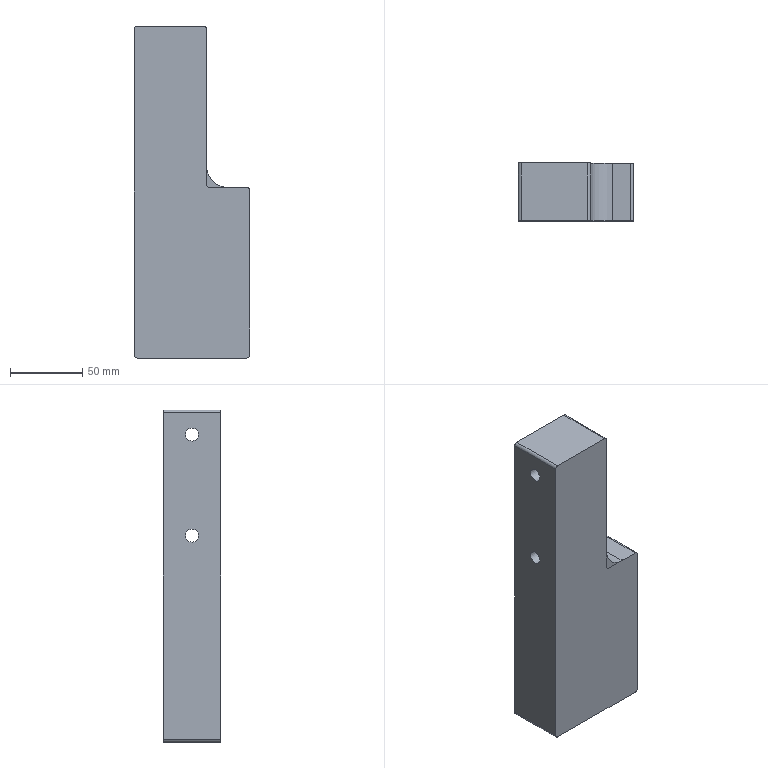NC program | NX | posted with a generic post | part box 80 x 40 x 230 mm
Whole program:
N10 G17 G21 G94 G90
(DRILLING , TOOL : D8点钻)
N12 T03 M6
N14 G54
N16 G17 G0 G90 X-67. Y-20.1 B0. C0. S1000 M3
N18 G43 Z20. H3
N20 G94 G81 G99 Z-1.5 F80. R3.
N22 X-17.
N24 G80
N26 G0 X-17. Y-20.1 Z20.
N28 M5
(DRILLING_1 , TOOL : Z6.8)
N30 T10 M6
N32 G54
N34 G17 G0 G90 X-67. Y-20.1 B0. C0. S1200 M3
N36 G43 Z20. H10
N38 G94 G83 G99 Z-30. F80. Q2. R3.
N40 X-17.
N42 G80
N44 G0 X-17. Y-20.1 Z20.
N46 M5
(PLANAR_MILL_1 , TOOL : D6.)
N48 T05 M6
N50 G54
N52 G17 G0 G90 X-19.911 Y-16.462 B0. C0. S3500 M3
N54 G43 Z20. H5
N56 Z1.
N58 G94 G1 X-20.696 Y-17.229 Z0.994 F1000.
N60 X-21.334 Y-18.334 Z0.988
N62 X-21.65 Y-19.571 Z0.981
N64 Y-20.629 Z0.975
N66 X-21.334 Y-21.866 Z0.969
N68 X-20.696 Y-22.971 Z0.962
N70 X-19.783 Y-23.862 Z0.955
N72 X-18.867 Y-24.392 Z0.95
N74 X-17.463 Y-24.757 Z0.942
N76 X-16.014 Y-24.675 Z0.935
N78 X-14.66 Y-24.153 Z0.927
N80 X-13.531 Y-23.241 Z0.919
N82 X-12.736 Y-22.028 Z0.912
N84 X-12.35 Y-20.629 Z0.904
N86 Y-19.571 Z0.899
N88 X-12.736 Y-18.172 Z0.891
N90 X-13.531 Y-16.959 Z0.883
N92 X-14.66 Y-16.047 Z0.876
N94 X-16.014 Y-15.525 Z0.868
N96 X-17.463 Y-15.443 Z0.861
N98 X-18.867 Y-15.808 Z0.853
N100 X-19.783 Y-16.338 Z0.848
N102 X-20.696 Y-17.229 Z0.841
N104 X-21.334 Y-18.334 Z0.834
N106 X-21.65 Y-19.571 Z0.827
N108 Y-20.629 Z0.822
N110 X-21.334 Y-21.866 Z0.815
N112 X-20.696 Y-22.971 Z0.809
N114 X-19.783 Y-23.862 Z0.802
N116 X-18.867 Y-24.392 Z0.796
N118 X-17.463 Y-24.757 Z0.789
N120 X-16.014 Y-24.675 Z0.781
N122 X-14.66 Y-24.153 Z0.774
N124 X-13.531 Y-23.241 Z0.766
N126 X-12.736 Y-22.028 Z0.758
N128 X-12.35 Y-20.629 Z0.751
N130 Y-19.571 Z0.745
N132 X-12.736 Y-18.172 Z0.738
N134 X-13.531 Y-16.959 Z0.73
N136 X-14.66 Y-16.047 Z0.722
N138 X-16.014 Y-15.525 Z0.715
N140 X-17.463 Y-15.443 Z0.707
N142 X-18.867 Y-15.808 Z0.7
N144 X-19.783 Y-16.338 Z0.694
N146 X-20.696 Y-17.229 Z0.687
N148 X-21.334 Y-18.334 Z0.681
N150 X-21.65 Y-19.571 Z0.674
N152 Y-20.629 Z0.668
N154 X-21.334 Y-21.866 Z0.662
N156 X-20.696 Y-22.971 Z0.655
N158 X-19.783 Y-23.862 Z0.648
N160 X-18.867 Y-24.392 Z0.643
N162 X-17.463 Y-24.757 Z0.635
N164 X-16.014 Y-24.675 Z0.628
N166 X-14.66 Y-24.153 Z0.62
N168 X-13.531 Y-23.241 Z0.613
N170 X-12.736 Y-22.028 Z0.605
N172 X-12.35 Y-20.629 Z0.597
N174 Y-19.571 Z0.592
N176 X-12.736 Y-18.172 Z0.584
N178 X-13.531 Y-16.959 Z0.577
N180 X-14.66 Y-16.047 Z0.569
N182 X-16.014 Y-15.525 Z0.561
N184 X-17.463 Y-15.443 Z0.554
N186 X-18.867 Y-15.808 Z0.546
N188 X-19.783 Y-16.338 Z0.541
N190 X-20.696 Y-17.229 Z0.534
N192 X-21.334 Y-18.334 Z0.527
N194 X-21.65 Y-19.571 Z0.521
N196 Y-20.629 Z0.515
N198 X-21.334 Y-21.866 Z0.508
N200 X-20.696 Y-22.971 Z0.502
N202 X-19.783 Y-23.862 Z0.495
N204 X-18.867 Y-24.392 Z0.489
N206 X-17.463 Y-24.757 Z0.482
N208 X-16.014 Y-24.675 Z0.474
N210 X-14.66 Y-24.153 Z0.467
N212 X-13.531 Y-23.241 Z0.459
N214 X-12.736 Y-22.028 Z0.451
N216 X-12.35 Y-20.629 Z0.444
N218 Y-19.571 Z0.438
N220 X-12.736 Y-18.172 Z0.431
N222 X-13.531 Y-16.959 Z0.423
N224 X-14.66 Y-16.047 Z0.416
N226 X-16.014 Y-15.525 Z0.408
N228 X-17.463 Y-15.443 Z0.4
N230 X-18.867 Y-15.808 Z0.393
N232 X-19.783 Y-16.338 Z0.387
N234 X-20.696 Y-17.229 Z0.381
N236 X-21.334 Y-18.334 Z0.374
N238 X-21.65 Y-19.571 Z0.367
N240 Y-20.629 Z0.362
N242 X-21.334 Y-21.866 Z0.355
N244 X-20.696 Y-22.971 Z0.348
N246 X-19.783 Y-23.862 Z0.342
N248 X-18.867 Y-24.392 Z0.336
N250 X-17.463 Y-24.757 Z0.328
N252 X-16.014 Y-24.675 Z0.321
N254 X-14.66 Y-24.153 Z0.313
N256 X-13.531 Y-23.241 Z0.306
N258 X-12.736 Y-22.028 Z0.298
N260 X-12.35 Y-20.629 Z0.29
N262 Y-19.571 Z0.285
N264 X-12.736 Y-18.172 Z0.277
N266 X-13.531 Y-16.959 Z0.27
N268 X-14.66 Y-16.047 Z0.262
N270 X-16.014 Y-15.525 Z0.255
N272 X-17.463 Y-15.443 Z0.247
N274 X-18.867 Y-15.808 Z0.239
N276 X-19.783 Y-16.338 Z0.234
N278 X-20.696 Y-17.229 Z0.227
N280 X-21.334 Y-18.334 Z0.22
N282 X-21.65 Y-19.571 Z0.214
N284 Y-20.629 Z0.208
N286 X-21.334 Y-21.866 Z0.202
N288 X-20.696 Y-22.971 Z0.195
N290 X-19.783 Y-23.862 Z0.188
N292 X-18.867 Y-24.392 Z0.183
N294 X-17.463 Y-24.757 Z0.175
N296 X-16.014 Y-24.675 Z0.167
N298 X-14.66 Y-24.153 Z0.16
N300 X-13.531 Y-23.241 Z0.152
N302 X-12.736 Y-22.028 Z0.145
N304 X-12.35 Y-20.629 Z0.137
N306 Y-19.571 Z0.132
N308 X-12.736 Y-18.172 Z0.124
N310 X-13.531 Y-16.959 Z0.116
N312 X-14.66 Y-16.047 Z0.109
N314 X-16.014 Y-15.525 Z0.101
N316 X-17.463 Y-15.443 Z0.094
N318 X-18.867 Y-15.808 Z0.086
N320 X-19.783 Y-16.338 Z0.08
N322 X-20.696 Y-17.229 Z0.074
N324 X-21.334 Y-18.334 Z0.067
N326 X-21.65 Y-19.571 Z0.06
N328 Y-20.629 Z0.055
N330 X-21.334 Y-21.866 Z0.048
N332 X-20.696 Y-22.971 Z0.041
N334 X-19.783 Y-23.862 Z0.035
N336 X-18.867 Y-24.392 Z0.029
N338 X-17.463 Y-24.757 Z0.022
N340 X-16.014 Y-24.675 Z0.014
N342 X-14.66 Y-24.153 Z0.006
N344 X-13.531 Y-23.241 Z-0.001
N346 X-12.736 Y-22.028 Z-0.009
N348 X-12.35 Y-20.629 Z-0.016
N350 Y-19.571 Z-0.022
N352 X-12.736 Y-18.172 Z-0.03
N354 X-13.531 Y-16.959 Z-0.037
N356 X-14.66 Y-16.047 Z-0.045
N358 X-16.014 Y-15.525 Z-0.052
N360 X-17.463 Y-15.443 Z-0.06
N362 X-18.867 Y-15.808 Z-0.068
N364 X-19.783 Y-16.338 Z-0.073
N366 X-20.696 Y-17.229 Z-0.08
N368 X-21.334 Y-18.334 Z-0.086
N370 X-21.65 Y-19.571 Z-0.093
N372 Y-20.629 Z-0.099
N374 X-21.334 Y-21.866 Z-0.105
N376 X-20.696 Y-22.971 Z-0.112
N378 X-19.783 Y-23.862 Z-0.119
N380 X-18.867 Y-24.392 Z-0.124
N382 X-17.463 Y-24.757 Z-0.132
N384 X-16.014 Y-24.675 Z-0.139
N386 X-14.66 Y-24.153 Z-0.147
N388 X-13.531 Y-23.241 Z-0.155
N390 X-12.736 Y-22.028 Z-0.162
N392 X-12.35 Y-20.629 Z-0.17
N394 Y-19.571 Z-0.175
N396 X-12.736 Y-18.172 Z-0.183
N398 X-13.531 Y-16.959 Z-0.191
N400 X-14.66 Y-16.047 Z-0.198
N402 X-16.014 Y-15.525 Z-0.206
N404 X-17.463 Y-15.443 Z-0.213
N406 X-18.867 Y-15.808 Z-0.221
N408 X-19.783 Y-16.338 Z-0.226
N410 X-20.696 Y-17.229 Z-0.233
N412 X-21.334 Y-18.334 Z-0.24
N414 X-21.65 Y-19.571 Z-0.247
N416 Y-20.629 Z-0.252
N418 X-21.334 Y-21.866 Z-0.259
N420 X-20.696 Y-22.971 Z-0.265
N422 X-19.783 Y-23.862 Z-0.272
N424 X-18.867 Y-24.392 Z-0.278
N426 X-17.463 Y-24.757 Z-0.285
N428 X-16.014 Y-24.675 Z-0.293
N430 X-14.66 Y-24.153 Z-0.3
N432 X-13.531 Y-23.241 Z-0.308
N434 X-12.736 Y-22.028 Z-0.316
N436 X-12.35 Y-20.629 Z-0.323
N438 Y-19.571 Z-0.329
N440 X-12.736 Y-18.172 Z-0.336
N442 X-13.531 Y-16.959 Z-0.344
N444 X-14.66 Y-16.047 Z-0.352
N446 X-16.014 Y-15.525 Z-0.359
N448 X-17.463 Y-15.443 Z-0.367
N450 X-18.867 Y-15.808 Z-0.374
N452 X-19.783 Y-16.338 Z-0.38
N454 X-20.696 Y-17.229 Z-0.387
N456 X-21.334 Y-18.334 Z-0.393
N458 X-21.65 Y-19.571 Z-0.4
N460 Y-20.629 Z-0.405
N462 X-21.334 Y-21.866 Z-0.412
N464 X-20.696 Y-22.971 Z-0.419
N466 X-19.783 Y-23.862 Z-0.426
N468 X-18.867 Y-24.392 Z-0.431
N470 X-17.463 Y-24.757 Z-0.439
N472 X-16.014 Y-24.675 Z-0.446
N474 X-14.66 Y-24.153 Z-0.454
N476 X-13.531 Y-23.241 Z-0.461
N478 X-12.736 Y-22.028 Z-0.469
N480 X-12.35 Y-20.629 Z-0.477
N482 Y-19.571 Z-0.482
N484 X-12.736 Y-18.172 Z-0.49
N486 X-13.531 Y-16.959 Z-0.497
N488 X-14.66 Y-16.047 Z-0.505
N490 X-16.014 Y-15.525 Z-0.513
N492 X-17.463 Y-15.443 Z-0.52
N494 X-18.867 Y-15.808 Z-0.528
N496 X-19.783 Y-16.338 Z-0.533
N498 X-20.696 Y-17.229 Z-0.54
N500 X-21.334 Y-18.334 Z-0.547
N502 X-21.65 Y-19.571 Z-0.553
N504 Y-20.629 Z-0.559
N506 X-21.334 Y-21.866 Z-0.566
N508 X-20.696 Y-22.971 Z-0.572
N510 X-19.783 Y-23.862 Z-0.579
N512 X-18.867 Y-24.392 Z-0.584
N514 X-17.463 Y-24.757 Z-0.592
N516 X-16.014 Y-24.675 Z-0.6
N518 X-14.66 Y-24.153 Z-0.607
N520 X-13.531 Y-23.241 Z-0.615
N522 X-12.736 Y-22.028 Z-0.622
N524 X-12.35 Y-20.629 Z-0.63
N526 Y-19.571 Z-0.636
N528 X-12.736 Y-18.172 Z-0.643
N530 X-13.531 Y-16.959 Z-0.651
N532 X-14.66 Y-16.047 Z-0.658
N534 X-16.014 Y-15.525 Z-0.666
N536 X-17.463 Y-15.443 Z-0.674
N538 X-18.867 Y-15.808 Z-0.681
N540 X-19.783 Y-16.338 Z-0.687
N542 X-20.696 Y-17.229 Z-0.693
N544 X-21.334 Y-18.334 Z-0.7
N546 X-21.65 Y-19.571 Z-0.707
N548 Y-20.629 Z-0.712
N550 X-21.334 Y-21.866 Z-0.719
N552 X-20.696 Y-22.971 Z-0.726
N554 X-19.783 Y-23.862 Z-0.732
N556 X-18.867 Y-24.392 Z-0.738
N558 X-17.463 Y-24.757 Z-0.746
N560 X-16.014 Y-24.675 Z-0.753
N562 X-14.66 Y-24.153 Z-0.761
N564 X-13.531 Y-23.241 Z-0.768
N566 X-12.736 Y-22.028 Z-0.776
N568 X-12.35 Y-20.629 Z-0.784
N570 Y-19.571 Z-0.789
N572 X-12.736 Y-18.172 Z-0.797
N574 X-13.531 Y-16.959 Z-0.804
N576 X-14.66 Y-16.047 Z-0.812
N578 X-16.014 Y-15.525 Z-0.819
N580 X-17.463 Y-15.443 Z-0.827
N582 X-18.867 Y-15.808 Z-0.835
N584 X-19.783 Y-16.338 Z-0.84
N586 X-20.696 Y-17.229 Z-0.847
N588 X-21.334 Y-18.334 Z-0.854
N590 X-21.65 Y-19.571 Z-0.86
N592 Y-20.629 Z-0.866
N594 X-21.334 Y-21.866 Z-0.872
N596 X-20.696 Y-22.971 Z-0.879
N598 X-19.783 Y-23.862 Z-0.886
N600 X-18.867 Y-24.392 Z-0.891
N602 X-17.463 Y-24.757 Z-0.899
N604 X-16.014 Y-24.675 Z-0.907
N606 X-14.66 Y-24.153 Z-0.914
N608 X-13.531 Y-23.241 Z-0.922
N610 X-12.736 Y-22.028 Z-0.929
N612 X-12.35 Y-20.629 Z-0.937
N614 Y-19.571 Z-0.942
N616 X-12.736 Y-18.172 Z-0.95
N618 X-13.531 Y-16.959 Z-0.958
N620 X-14.66 Y-16.047 Z-0.965
N622 X-16.014 Y-15.525 Z-0.973
N624 X-17.463 Y-15.443 Z-0.98
N626 X-18.867 Y-15.808 Z-0.988
N628 X-19.783 Y-16.338 Z-0.994
N630 X-20.696 Y-17.229 Z-1.
N632 X-21.334 Y-18.334 Z-1.007
N634 X-21.65 Y-19.571 Z-1.014
N636 Y-20.629 Z-1.019
N638 X-21.334 Y-21.866 Z-1.026
N640 X-20.696 Y-22.971 Z-1.033
N642 X-19.783 Y-23.862 Z-1.039
N644 X-18.867 Y-24.392 Z-1.045
N646 X-17.463 Y-24.757 Z-1.052
N648 X-16.014 Y-24.675 Z-1.06
N650 X-14.66 Y-24.153 Z-1.068
N652 X-13.531 Y-23.241 Z-1.075
N654 X-12.736 Y-22.028 Z-1.083
N656 X-12.35 Y-20.629 Z-1.09
N658 Y-19.571 Z-1.096
N660 X-12.736 Y-18.172 Z-1.103
N662 X-13.531 Y-16.959 Z-1.111
N664 X-14.66 Y-16.047 Z-1.119
N666 X-16.014 Y-15.525 Z-1.126
N668 X-17.463 Y-15.443 Z-1.134
N670 X-18.867 Y-15.808 Z-1.141
N672 X-19.783 Y-16.338 Z-1.147
N674 X-20.696 Y-17.229 Z-1.154
N676 X-21.334 Y-18.334 Z-1.16
N678 X-21.65 Y-19.571 Z-1.167
N680 Y-20.629 Z-1.173
N682 X-21.334 Y-21.866 Z-1.179
N684 X-20.696 Y-22.971 Z-1.186
N686 X-19.783 Y-23.862 Z-1.193
N688 X-18.867 Y-24.392 Z-1.198
N690 X-17.463 Y-24.757 Z-1.206
N692 X-16.014 Y-24.675 Z-1.213
N694 X-14.66 Y-24.153 Z-1.221
N696 X-13.531 Y-23.241 Z-1.229
N698 X-12.736 Y-22.028 Z-1.236
N700 X-12.35 Y-20.629 Z-1.244
N702 Y-19.571 Z-1.249
N704 X-12.736 Y-18.172 Z-1.257
N706 X-13.531 Y-16.959 Z-1.265
N708 X-14.66 Y-16.047 Z-1.272
N710 X-16.014 Y-15.525 Z-1.28
N712 X-17.463 Y-15.443 Z-1.287
N714 X-18.867 Y-15.808 Z-1.295
N716 X-19.783 Y-16.338 Z-1.3
N718 X-20.696 Y-17.229 Z-1.307
N720 X-21.334 Y-18.334 Z-1.314
N722 X-21.65 Y-19.571 Z-1.32
N724 Y-20.629 Z-1.326
N726 X-21.334 Y-21.866 Z-1.333
N728 X-20.696 Y-22.971 Z-1.339
N730 X-19.783 Y-23.862 Z-1.346
N732 X-18.867 Y-24.392 Z-1.352
N734 X-17.463 Y-24.757 Z-1.359
N736 X-16.014 Y-24.675 Z-1.367
N738 X-14.66 Y-24.153 Z-1.374
N740 X-13.531 Y-23.241 Z-1.382
N742 X-12.736 Y-22.028 Z-1.39
N744 X-12.35 Y-20.629 Z-1.397
N746 Y-19.571 Z-1.403
N748 X-12.736 Y-18.172 Z-1.41
N750 X-13.531 Y-16.959 Z-1.418
N752 X-14.66 Y-16.047 Z-1.426
N754 X-16.014 Y-15.525 Z-1.433
N756 X-17.463 Y-15.443 Z-1.441
N758 X-18.867 Y-15.808 Z-1.448
N760 X-19.783 Y-16.338 Z-1.454
N762 X-20.696 Y-17.229 Z-1.461
N764 X-21.334 Y-18.334 Z-1.467
N766 X-21.65 Y-19.571 Z-1.474
N768 Y-20.629 Z-1.479
N770 X-21.334 Y-21.866 Z-1.486
N772 X-20.696 Y-22.971 Z-1.493
N774 X-19.783 Y-23.862 Z-1.5
N776 X-18.867 Y-24.392 Z-1.505
N778 X-17.463 Y-24.757 Z-1.513
N780 X-16.014 Y-24.675 Z-1.52
N782 X-14.66 Y-24.153 Z-1.528
N784 X-13.531 Y-23.241 Z-1.535
N786 X-12.736 Y-22.028 Z-1.543
N788 X-12.35 Y-20.629 Z-1.551
N790 Y-19.571 Z-1.556
N792 X-12.736 Y-18.172 Z-1.564
N794 X-13.531 Y-16.959 Z-1.571
N796 X-14.66 Y-16.047 Z-1.579
N798 X-16.014 Y-15.525 Z-1.587
N800 X-17.463 Y-15.443 Z-1.594
N802 X-18.867 Y-15.808 Z-1.602
N804 X-19.783 Y-16.338 Z-1.607
N806 X-20.696 Y-17.229 Z-1.614
N808 X-21.334 Y-18.334 Z-1.621
N810 X-21.65 Y-19.571 Z-1.627
N812 Y-20.629 Z-1.633
N814 X-21.334 Y-21.866 Z-1.64
N816 X-20.696 Y-22.971 Z-1.646
N818 X-19.783 Y-23.862 Z-1.653
N820 X-18.867 Y-24.392 Z-1.658
N822 X-17.463 Y-24.757 Z-1.666
N824 X-16.014 Y-24.675 Z-1.674
N826 X-14.66 Y-24.153 Z-1.681
N828 X-13.531 Y-23.241 Z-1.689
N830 X-12.736 Y-22.028 Z-1.696
N832 X-12.35 Y-20.629 Z-1.704
N834 Y-19.571 Z-1.71
N836 X-12.736 Y-18.172 Z-1.717
N838 X-13.531 Y-16.959 Z-1.725
N840 X-14.66 Y-16.047 Z-1.732
N842 X-16.014 Y-15.525 Z-1.74
N844 X-17.463 Y-15.443 Z-1.748
N846 X-18.867 Y-15.808 Z-1.755
N848 X-19.783 Y-16.338 Z-1.761
N850 X-20.696 Y-17.229 Z-1.767
N852 X-21.334 Y-18.334 Z-1.774
N854 X-21.65 Y-19.571 Z-1.781
N856 Y-20.629 Z-1.786
N858 X-21.334 Y-21.866 Z-1.793
N860 X-20.696 Y-22.971 Z-1.8
N862 X-19.783 Y-23.862 Z-1.806
N864 X-18.867 Y-24.392 Z-1.812
N866 X-17.463 Y-24.757 Z-1.819
N868 X-16.014 Y-24.675 Z-1.827
N870 X-14.66 Y-24.153 Z-1.835
N872 X-13.531 Y-23.241 Z-1.842
N874 X-12.736 Y-22.028 Z-1.85
N876 X-12.35 Y-20.629 Z-1.857
N878 Y-19.571 Z-1.863
N880 X-12.736 Y-18.172 Z-1.871
N882 X-13.531 Y-16.959 Z-1.878
N884 X-14.66 Y-16.047 Z-1.886
N886 X-16.014 Y-15.525 Z-1.893
N888 X-17.463 Y-15.443 Z-1.901
N890 X-18.867 Y-15.808 Z-1.909
N892 X-19.783 Y-16.338 Z-1.914
N894 X-20.696 Y-17.229 Z-1.921
N896 X-21.334 Y-18.334 Z-1.928
N898 X-21.65 Y-19.571 Z-1.934
N900 Y-20.629 Z-1.94
N902 X-21.334 Y-21.866 Z-1.946
N904 X-20.696 Y-22.971 Z-1.953
N906 X-19.783 Y-23.862 Z-1.96
N908 X-18.867 Y-24.392 Z-1.965
N910 X-17.463 Y-24.757 Z-1.973
N912 X-16.014 Y-24.675 Z-1.981
N914 X-14.66 Y-24.153 Z-1.988
N916 X-13.531 Y-23.241 Z-1.996
N918 X-12.736 Y-22.028 Z-2.003
N920 X-12.35 Y-20.629 Z-2.011
N922 Y-19.571 Z-2.016
N924 X-12.736 Y-18.172 Z-2.024
N926 X-13.531 Y-16.959 Z-2.032
N928 X-14.66 Y-16.047 Z-2.039
N930 X-16.014 Y-15.525 Z-2.047
N932 X-17.463 Y-15.443 Z-2.054
N934 X-18.867 Y-15.808 Z-2.062
N936 X-19.783 Y-16.338 Z-2.068
N938 X-20.696 Y-17.229 Z-2.074
N940 X-21.334 Y-18.334 Z-2.081
N942 X-21.65 Y-19.571 Z-2.088
N944 Y-20.629 Z-2.093
N946 X-21.334 Y-21.866 Z-2.1
N948 X-20.696 Y-22.971 Z-2.107
N950 X-19.783 Y-23.862 Z-2.113
N952 X-18.867 Y-24.392 Z-2.119
N954 X-17.463 Y-24.757 Z-2.126
N956 X-16.014 Y-24.675 Z-2.134
N958 X-14.66 Y-24.153 Z-2.142
N960 X-13.531 Y-23.241 Z-2.149
N962 X-12.736 Y-22.028 Z-2.157
N964 X-12.35 Y-20.629 Z-2.164
N966 Y-19.571 Z-2.17
N968 X-12.736 Y-18.172 Z-2.177
N970 X-13.531 Y-16.959 Z-2.185
N972 X-14.66 Y-16.047 Z-2.193
N974 X-16.014 Y-15.525 Z-2.2
N976 X-17.463 Y-15.443 Z-2.208
N978 X-18.867 Y-15.808 Z-2.215
N980 X-19.783 Y-16.338 Z-2.221
N982 X-20.696 Y-17.229 Z-2.228
N984 X-21.334 Y-18.334 Z-2.234
N986 X-21.65 Y-19.571 Z-2.241
N988 Y-20.629 Z-2.247
N990 X-21.334 Y-21.866 Z-2.253
N992 X-20.696 Y-22.971 Z-2.26
N994 X-19.783 Y-23.862 Z-2.267
N996 X-18.867 Y-24.392 Z-2.272
N998 X-17.463 Y-24.757 Z-2.28
N1000 X-16.014 Y-24.675 Z-2.287
N1002 X-14.66 Y-24.153 Z-2.295
N1004 X-13.531 Y-23.241 Z-2.303
N1006 X-12.736 Y-22.028 Z-2.31
N1008 X-12.35 Y-20.629 Z-2.318
N1010 Y-19.571 Z-2.323
N1012 X-12.736 Y-18.172 Z-2.331
N1014 X-13.531 Y-16.959 Z-2.338
N1016 X-14.66 Y-16.047 Z-2.346
N1018 X-16.014 Y-15.525 Z-2.354
N1020 X-17.463 Y-15.443 Z-2.361
N1022 X-18.867 Y-15.808 Z-2.369
N1024 X-19.783 Y-16.338 Z-2.374
N1026 X-20.696 Y-17.229 Z-2.381
N1028 X-21.334 Y-18.334 Z-2.388
N1030 X-21.65 Y-19.571 Z-2.394
N1032 Y-20.629 Z-2.4
N1034 X-21.334 Y-21.866 Z-2.407
N1036 X-20.696 Y-22.971 Z-2.413
N1038 X-19.783 Y-23.862 Z-2.42
N1040 X-18.867 Y-24.392 Z-2.426
N1042 X-17.463 Y-24.757 Z-2.433
N1044 X-16.014 Y-24.675 Z-2.441
N1046 X-14.66 Y-24.153 Z-2.448
N1048 X-13.531 Y-23.241 Z-2.456
N1050 X-12.736 Y-22.028 Z-2.464
N1052 X-12.35 Y-20.629 Z-2.471
N1054 Y-19.571 Z-2.477
N1056 X-12.736 Y-18.172 Z-2.484
N1058 X-13.531 Y-16.959 Z-2.492
N1060 X-14.66 Y-16.047 Z-2.5
N1062 X-16.014 Y-15.525 Z-2.507
N1064 X-17.463 Y-15.443 Z-2.515
N1066 X-18.867 Y-15.808 Z-2.522
N1068 X-19.783 Y-16.338 Z-2.528
N1070 X-20.696 Y-17.229 Z-2.535
N1072 X-21.334 Y-18.334 Z-2.541
N1074 X-21.65 Y-19.571 Z-2.548
N1076 Y-20.629 Z-2.553
N1078 X-21.334 Y-21.866 Z-2.56
N1080 X-20.696 Y-22.971 Z-2.567
N1082 X-19.783 Y-23.862 Z-2.573
N1084 X-18.867 Y-24.392 Z-2.579
N1086 X-17.463 Y-24.757 Z-2.587
N1088 X-16.014 Y-24.675 Z-2.594
N1090 X-14.66 Y-24.153 Z-2.602
N1092 X-13.531 Y-23.241 Z-2.609
N1094 X-12.736 Y-22.028 Z-2.617
N1096 X-12.35 Y-20.629 Z-2.625
N1098 Y-19.571 Z-2.63
N1100 X-12.736 Y-18.172 Z-2.638
N1102 X-13.531 Y-16.959 Z-2.645
N1104 X-14.66 Y-16.047 Z-2.653
N1106 X-16.014 Y-15.525 Z-2.661
N1108 X-17.463 Y-15.443 Z-2.668
N1110 X-18.867 Y-15.808 Z-2.676
N1112 X-19.783 Y-16.338 Z-2.681
N1114 X-20.696 Y-17.229 Z-2.688
N1116 X-21.334 Y-18.334 Z-2.695
N1118 X-21.65 Y-19.571 Z-2.701
N1120 Y-20.629 Z-2.707
N1122 X-21.334 Y-21.866 Z-2.714
N1124 X-20.696 Y-22.971 Z-2.72
N1126 X-19.783 Y-23.862 Z-2.727
N1128 X-18.867 Y-24.392 Z-2.732
N1130 X-17.463 Y-24.757 Z-2.74
N1132 X-16.014 Y-24.675 Z-2.748
N1134 X-14.66 Y-24.153 Z-2.755
N1136 X-13.531 Y-23.241 Z-2.763
N1138 X-12.736 Y-22.028 Z-2.77
N1140 X-12.35 Y-20.629 Z-2.778
N1142 Y-19.571 Z-2.784
N1144 X-12.736 Y-18.172 Z-2.791
N1146 X-13.531 Y-16.959 Z-2.799
N1148 X-14.66 Y-16.047 Z-2.806
N1150 X-16.014 Y-15.525 Z-2.814
N1152 X-17.463 Y-15.443 Z-2.822
N1154 X-18.867 Y-15.808 Z-2.829
N1156 X-19.783 Y-16.338 Z-2.835
N1158 X-20.696 Y-17.229 Z-2.841
N1160 X-21.334 Y-18.334 Z-2.848
N1162 X-21.65 Y-19.571 Z-2.855
N1164 Y-20.629 Z-2.86
N1166 X-21.334 Y-21.866 Z-2.867
N1168 X-20.696 Y-22.971 Z-2.874
N1170 X-19.783 Y-23.862 Z-2.88
N1172 X-18.867 Y-24.392 Z-2.886
N1174 X-17.463 Y-24.757 Z-2.893
N1176 X-16.014 Y-24.675 Z-2.901
N1178 X-14.66 Y-24.153 Z-2.909
N1180 X-13.531 Y-23.241 Z-2.916
N1182 X-12.736 Y-22.028 Z-2.924
N1184 X-12.35 Y-20.629 Z-2.931
N1186 Y-19.571 Z-2.937
N1188 X-12.736 Y-18.172 Z-2.945
N1190 X-13.531 Y-16.959 Z-2.952
N1192 X-14.66 Y-16.047 Z-2.96
N1194 X-16.014 Y-15.525 Z-2.967
N1196 X-17.463 Y-15.443 Z-2.975
N1198 X-18.867 Y-15.808 Z-2.983
N1200 X-19.783 Y-16.338 Z-2.988
N1202 X-20.696 Y-17.229 Z-2.995
N1204 X-21.334 Y-18.334 Z-3.001
N1206 X-21.65 Y-19.571 Z-3.008
N1208 Y-20.629 Z-3.014
N1210 X-21.334 Y-21.866 Z-3.02
N1212 X-20.696 Y-22.971 Z-3.027
N1214 X-19.783 Y-23.862 Z-3.034
N1216 X-18.867 Y-24.392 Z-3.039
N1218 X-17.463 Y-24.757 Z-3.047
N1220 X-16.014 Y-24.675 Z-3.054
N1222 X-14.66 Y-24.153 Z-3.062
N1224 X-13.531 Y-23.241 Z-3.07
N1226 X-12.736 Y-22.028 Z-3.077
N1228 X-12.35 Y-20.629 Z-3.085
N1230 Y-19.571 Z-3.09
N1232 X-12.736 Y-18.172 Z-3.098
N1234 X-13.531 Y-16.959 Z-3.106
N1236 X-14.66 Y-16.047 Z-3.113
N1238 X-16.014 Y-15.525 Z-3.121
N1240 X-17.463 Y-15.443 Z-3.128
N1242 X-18.867 Y-15.808 Z-3.136
N1244 X-19.783 Y-16.338 Z-3.142
N1246 X-20.696 Y-17.229 Z-3.148
N1248 X-21.334 Y-18.334 Z-3.155
N1250 X-21.65 Y-19.571 Z-3.162
N1252 Y-20.629 Z-3.167
N1254 X-21.334 Y-21.866 Z-3.174
N1256 X-20.696 Y-22.971 Z-3.181
N1258 X-19.783 Y-23.862 Z-3.187
N1260 X-18.867 Y-24.392 Z-3.193
N1262 X-17.463 Y-24.757 Z-3.2
N1264 X-16.014 Y-24.675 Z-3.208
N1266 X-14.66 Y-24.153 Z-3.216
N1268 X-13.531 Y-23.241 Z-3.223
N1270 X-12.736 Y-22.028 Z-3.231
N1272 X-12.35 Y-20.629 Z-3.238
N1274 Y-19.571 Z-3.244
N1276 X-12.736 Y-18.172 Z-3.251
N1278 X-13.531 Y-16.959 Z-3.259
N1280 X-14.66 Y-16.047 Z-3.267
N1282 X-16.014 Y-15.525 Z-3.274
N1284 X-17.463 Y-15.443 Z-3.282
N1286 X-18.867 Y-15.808 Z-3.289
N1288 X-19.783 Y-16.338 Z-3.295
N1290 X-20.696 Y-17.229 Z-3.302
N1292 X-21.334 Y-18.334 Z-3.308
N1294 X-21.65 Y-19.571 Z-3.315
N1296 Y-20.629 Z-3.321
N1298 X-21.334 Y-21.866 Z-3.327
N1300 X-20.696 Y-22.971 Z-3.334
N1302 X-19.783 Y-23.862 Z-3.341
N1304 X-18.867 Y-24.392 Z-3.346
N1306 X-17.463 Y-24.757 Z-3.354
N1308 X-16.014 Y-24.675 Z-3.361
N1310 X-14.66 Y-24.153 Z-3.369
N1312 X-13.531 Y-23.241 Z-3.377
N1314 X-12.736 Y-22.028 Z-3.384
N1316 X-12.35 Y-20.629 Z-3.392
N1318 Y-19.571 Z-3.397
N1320 X-12.736 Y-18.172 Z-3.405
N1322 X-13.531 Y-16.959 Z-3.412
N1324 X-14.66 Y-16.047 Z-3.42
N1326 X-16.014 Y-15.525 Z-3.428
N1328 X-17.463 Y-15.443 Z-3.435
N1330 X-18.867 Y-15.808 Z-3.443
N1332 X-19.783 Y-16.338 Z-3.448
N1334 X-20.696 Y-17.229 Z-3.455
N1336 X-21.334 Y-18.334 Z-3.462
N1338 X-21.65 Y-19.571 Z-3.468
N1340 Y-20.629 Z-3.474
N1342 X-21.334 Y-21.866 Z-3.481
N1344 X-20.696 Y-22.971 Z-3.487
N1346 X-19.783 Y-23.862 Z-3.494
N1348 X-18.867 Y-24.392 Z-3.5
N1350 X-17.463 Y-24.757 Z-3.507
N1352 X-16.014 Y-24.675 Z-3.515
N1354 X-14.66 Y-24.153 Z-3.522
N1356 X-13.531 Y-23.241 Z-3.53
N1358 X-12.736 Y-22.028 Z-3.538
N1360 X-12.35 Y-20.629 Z-3.545
N1362 Y-19.571 Z-3.551
N1364 X-12.736 Y-18.172 Z-3.558
N1366 X-13.531 Y-16.959 Z-3.566
N1368 X-14.66 Y-16.047 Z-3.573
N1370 X-16.014 Y-15.525 Z-3.581
N1372 X-17.463 Y-15.443 Z-3.589
N1374 X-18.867 Y-15.808 Z-3.596
N1376 X-19.783 Y-16.338 Z-3.602
N1378 X-20.696 Y-17.229 Z-3.609
N1380 X-21.334 Y-18.334 Z-3.615
N1382 X-21.65 Y-19.571 Z-3.622
N1384 Y-20.629 Z-3.627
N1386 X-21.334 Y-21.866 Z-3.634
N1388 X-20.696 Y-22.971 Z-3.641
N1390 X-19.783 Y-23.862 Z-3.647
N1392 X-18.867 Y-24.392 Z-3.653
N1394 X-17.463 Y-24.757 Z-3.661
N1396 X-16.014 Y-24.675 Z-3.668
N1398 X-14.66 Y-24.153 Z-3.676
N1400 X-13.531 Y-23.241 Z-3.683
N1402 X-12.736 Y-22.028 Z-3.691
N1404 X-12.35 Y-20.629 Z-3.699
N1406 Y-19.571 Z-3.704
N1408 X-12.736 Y-18.172 Z-3.712
N1410 X-13.531 Y-16.959 Z-3.719
N1412 X-14.66 Y-16.047 Z-3.727
N1414 X-16.014 Y-15.525 Z-3.735
N1416 X-17.463 Y-15.443 Z-3.742
N1418 X-18.867 Y-15.808 Z-3.75
N1420 X-19.783 Y-16.338 Z-3.755
N1422 X-20.696 Y-17.229 Z-3.762
N1424 X-21.334 Y-18.334 Z-3.769
N1426 X-21.65 Y-19.571 Z-3.775
N1428 Y-20.629 Z-3.781
N1430 X-21.334 Y-21.866 Z-3.788
N1432 X-20.696 Y-22.971 Z-3.794
N1434 X-19.783 Y-23.862 Z-3.801
N1436 X-18.867 Y-24.392 Z-3.806
N1438 X-17.463 Y-24.757 Z-3.814
N1440 X-16.014 Y-24.675 Z-3.822
N1442 X-14.66 Y-24.153 Z-3.829
N1444 X-13.531 Y-23.241 Z-3.837
N1446 X-12.736 Y-22.028 Z-3.844
N1448 X-12.35 Y-20.629 Z-3.852
N1450 Y-19.571 Z-3.858
N1452 X-12.736 Y-18.172 Z-3.865
N1454 X-13.531 Y-16.959 Z-3.873
N1456 X-14.66 Y-16.047 Z-3.88
N1458 X-16.014 Y-15.525 Z-3.888
N1460 X-17.463 Y-15.443 Z-3.896
N1462 X-18.867 Y-15.808 Z-3.903
N1464 X-19.783 Y-16.338 Z-3.909
N1466 X-20.696 Y-17.229 Z-3.915
N1468 X-21.334 Y-18.334 Z-3.922
N1470 X-21.65 Y-19.571 Z-3.929
N1472 Y-20.629 Z-3.934
N1474 X-21.334 Y-21.866 Z-3.941
N1476 X-20.696 Y-22.971 Z-3.948
N1478 X-19.783 Y-23.862 Z-3.954
N1480 X-18.867 Y-24.392 Z-3.96
N1482 X-17.463 Y-24.757 Z-3.967
N1484 X-16.014 Y-24.675 Z-3.975
N1486 X-14.66 Y-24.153 Z-3.983
N1488 X-13.531 Y-23.241 Z-3.99
N1490 X-12.736 Y-22.028 Z-3.998
N1492 X-12.35 Y-20.629 Z-4.005
N1494 Y-19.571 Z-4.011
N1496 X-12.736 Y-18.172 Z-4.019
N1498 X-13.531 Y-16.959 Z-4.026
N1500 X-14.66 Y-16.047 Z-4.034
N1502 X-16.014 Y-15.525 Z-4.041
N1504 X-17.463 Y-15.443 Z-4.049
N1506 X-18.867 Y-15.808 Z-4.057
N1508 X-19.783 Y-16.338 Z-4.062
N1510 X-20.696 Y-17.229 Z-4.069
N1512 X-21.334 Y-18.334 Z-4.075
N1514 X-21.65 Y-19.571 Z-4.082
N1516 Y-20.629 Z-4.088
N1518 X-21.334 Y-21.866 Z-4.094
N1520 X-20.696 Y-22.971 Z-4.101
N1522 X-19.783 Y-23.862 Z-4.108
N1524 X-18.867 Y-24.392 Z-4.113
N1526 X-17.463 Y-24.757 Z-4.121
N1528 X-16.014 Y-24.675 Z-4.128
N1530 X-14.66 Y-24.153 Z-4.136
N1532 X-13.531 Y-23.241 Z-4.144
N1534 X-12.736 Y-22.028 Z-4.151
N1536 X-12.35 Y-20.629 Z-4.159
N1538 Y-19.571 Z-4.164
N1540 X-12.736 Y-18.172 Z-4.172
N1542 X-13.531 Y-16.959 Z-4.18
N1544 X-14.66 Y-16.047 Z-4.187
N1546 X-16.014 Y-15.525 Z-4.195
N1548 X-17.463 Y-15.443 Z-4.202
N1550 X-18.867 Y-15.808 Z-4.21
N1552 X-19.783 Y-16.338 Z-4.216
N1554 X-20.696 Y-17.229 Z-4.222
N1556 X-21.334 Y-18.334 Z-4.229
N1558 X-21.65 Y-19.571 Z-4.236
N1560 Y-20.629 Z-4.241
N1562 X-21.334 Y-21.866 Z-4.248
N1564 X-20.696 Y-22.971 Z-4.254
N1566 X-19.783 Y-23.862 Z-4.261
N1568 X-18.867 Y-24.392 Z-4.267
N1570 X-17.463 Y-24.757 Z-4.274
N1572 X-16.014 Y-24.675 Z-4.282
N1574 X-14.66 Y-24.153 Z-4.289
N1576 X-13.531 Y-23.241 Z-4.297
N1578 X-12.736 Y-22.028 Z-4.305
N1580 X-12.35 Y-20.629 Z-4.312
N1582 Y-19.571 Z-4.318
N1584 X-12.736 Y-18.172 Z-4.325
N1586 X-13.531 Y-16.959 Z-4.333
N1588 X-14.66 Y-16.047 Z-4.341
N1590 X-16.014 Y-15.525 Z-4.348
N1592 X-17.463 Y-15.443 Z-4.356
N1594 X-18.867 Y-15.808 Z-4.363
N1596 X-19.783 Y-16.338 Z-4.369
N1598 X-20.696 Y-17.229 Z-4.376
N1600 X-21.334 Y-18.334 Z-4.382
N1602 X-21.65 Y-19.571 Z-4.389
N1604 Y-20.629 Z-4.395
N1606 X-21.334 Y-21.866 Z-4.401
N1608 X-20.696 Y-22.971 Z-4.408
N1610 X-19.783 Y-23.862 Z-4.415
N1612 X-18.867 Y-24.392 Z-4.42
N1614 X-17.463 Y-24.757 Z-4.428
N1616 X-16.014 Y-24.675 Z-4.435
N1618 X-14.66 Y-24.153 Z-4.443
N1620 X-13.531 Y-23.241 Z-4.451
N1622 X-12.736 Y-22.028 Z-4.458
N1624 X-12.35 Y-20.629 Z-4.466
N1626 Y-19.571 Z-4.471
N1628 X-12.736 Y-18.172 Z-4.479
N1630 X-13.531 Y-16.959 Z-4.486
N1632 X-14.66 Y-16.047 Z-4.494
N1634 X-16.014 Y-15.525 Z-4.502
N1636 X-17.463 Y-15.443 Z-4.509
N1638 X-18.867 Y-15.808 Z-4.517
N1640 X-19.783 Y-16.338 Z-4.522
N1642 X-20.696 Y-17.229 Z-4.529
N1644 X-21.334 Y-18.334 Z-4.536
N1646 X-21.65 Y-19.571 Z-4.542
N1648 Y-20.629 Z-4.548
N1650 X-21.334 Y-21.866 Z-4.555
N1652 X-20.696 Y-22.971 Z-4.561
N1654 X-19.783 Y-23.862 Z-4.568
N1656 X-18.867 Y-24.392 Z-4.574
N1658 X-17.463 Y-24.757 Z-4.581
N1660 X-16.014 Y-24.675 Z-4.589
N1662 X-14.66 Y-24.153 Z-4.596
N1664 X-13.531 Y-23.241 Z-4.604
N1666 X-12.736 Y-22.028 Z-4.612
N1668 X-12.35 Y-20.629 Z-4.619
N1670 Y-19.571 Z-4.625
N1672 X-12.736 Y-18.172 Z-4.632
N1674 X-13.531 Y-16.959 Z-4.64
N1676 X-14.66 Y-16.047 Z-4.647
N1678 X-16.014 Y-15.525 Z-4.655
N1680 X-17.463 Y-15.443 Z-4.663
N1682 X-18.867 Y-15.808 Z-4.67
N1684 X-19.783 Y-16.338 Z-4.676
N1686 X-20.696 Y-17.229 Z-4.682
N1688 X-21.334 Y-18.334 Z-4.689
N1690 X-21.65 Y-19.571 Z-4.696
N1692 Y-20.629 Z-4.701
N1694 X-21.334 Y-21.866 Z-4.708
N1696 X-20.696 Y-22.971 Z-4.715
N1698 X-19.783 Y-23.862 Z-4.721
N1700 X-18.867 Y-24.392 Z-4.727
N1702 X-17.463 Y-24.757 Z-4.735
N1704 X-16.014 Y-24.675 Z-4.742
N1706 X-14.66 Y-24.153 Z-4.75
N1708 X-13.531 Y-23.241 Z-4.757
N1710 X-12.736 Y-22.028 Z-4.765
N1712 X-12.35 Y-20.629 Z-4.773
N1714 Y-19.571 Z-4.778
N1716 X-12.736 Y-18.172 Z-4.786
N1718 X-13.531 Y-16.959 Z-4.793
N1720 X-14.66 Y-16.047 Z-4.801
N1722 X-16.014 Y-15.525 Z-4.808
N1724 X-17.463 Y-15.443 Z-4.816
N1726 X-18.867 Y-15.808 Z-4.824
N1728 X-19.783 Y-16.338 Z-4.829
N1730 X-20.696 Y-17.229 Z-4.836
N1732 X-21.334 Y-18.334 Z-4.843
N1734 X-21.65 Y-19.571 Z-4.849
N1736 Y-20.629 Z-4.855
N1738 X-21.334 Y-21.866 Z-4.861
N1740 X-20.696 Y-22.971 Z-4.868
N1742 X-19.783 Y-23.862 Z-4.875
N1744 X-18.867 Y-24.392 Z-4.88
N1746 X-17.463 Y-24.757 Z-4.888
N1748 X-16.014 Y-24.675 Z-4.896
N1750 X-14.66 Y-24.153 Z-4.903
N1752 X-13.531 Y-23.241 Z-4.911
N1754 X-12.736 Y-22.028 Z-4.918
N1756 X-12.35 Y-20.629 Z-4.926
N1758 Y-19.571 Z-4.932
N1760 X-12.736 Y-18.172 Z-4.939
N1762 X-13.531 Y-16.959 Z-4.947
N1764 X-14.66 Y-16.047 Z-4.954
N1766 X-16.014 Y-15.525 Z-4.962
N1768 X-17.463 Y-15.443 Z-4.97
N1770 X-18.867 Y-15.808 Z-4.977
N1772 X-19.783 Y-16.338 Z-4.983
N1774 X-20.696 Y-17.229 Z-4.989
N1776 X-21.334 Y-18.334 Z-4.996
N1778 X-21.65 Y-19.571 Z-5.003
N1780 Y-20.629 Z-5.008
N1782 X-21.334 Y-21.866 Z-5.015
N1784 X-20.696 Y-22.971 Z-5.022
N1786 X-19.783 Y-23.862 Z-5.028
N1788 X-18.867 Y-24.392 Z-5.034
N1790 X-17.463 Y-24.757 Z-5.041
N1792 X-16.014 Y-24.675 Z-5.049
N1794 X-14.66 Y-24.153 Z-5.057
N1796 X-13.531 Y-23.241 Z-5.064
N1798 X-12.736 Y-22.028 Z-5.072
N1800 X-12.35 Y-20.629 Z-5.079
N1802 Y-19.571 Z-5.085
N1804 X-12.736 Y-18.172 Z-5.093
N1806 X-13.531 Y-16.959 Z-5.1
N1808 X-14.66 Y-16.047 Z-5.108
N1810 X-16.014 Y-15.525 Z-5.115
N1812 X-17.463 Y-15.443 Z-5.123
N1814 X-18.867 Y-15.808 Z-5.131
N1816 X-19.783 Y-16.338 Z-5.136
N1818 X-20.696 Y-17.229 Z-5.143
N1820 X-21.334 Y-18.334 Z-5.149
N1822 X-21.65 Y-19.571 Z-5.156
N1824 Y-20.629 Z-5.162
N1826 X-21.334 Y-21.866 Z-5.168
N1828 X-20.696 Y-22.971 Z-5.175
N1830 X-19.783 Y-23.862 Z-5.182
N1832 X-18.867 Y-24.392 Z-5.187
N1834 X-17.463 Y-24.757 Z-5.195
N1836 X-16.014 Y-24.675 Z-5.202
N1838 X-14.66 Y-24.153 Z-5.21
N1840 X-13.531 Y-23.241 Z-5.218
N1842 X-12.736 Y-22.028 Z-5.225
N1844 X-12.35 Y-20.629 Z-5.233
N1846 Y-19.571 Z-5.238
N1848 X-12.736 Y-18.172 Z-5.246
N1850 X-13.531 Y-16.959 Z-5.254
N1852 X-14.66 Y-16.047 Z-5.261
N1854 X-16.014 Y-15.525 Z-5.269
N1856 X-17.463 Y-15.443 Z-5.276
N1858 X-18.867 Y-15.808 Z-5.284
N1860 X-19.783 Y-16.338 Z-5.29
N1862 X-20.696 Y-17.229 Z-5.296
N1864 X-21.334 Y-18.334 Z-5.303
N1866 X-21.65 Y-19.571 Z-5.31
N1868 Y-20.629 Z-5.315
N1870 X-21.334 Y-21.866 Z-5.322
N1872 X-20.696 Y-22.971 Z-5.328
N1874 X-19.783 Y-23.862 Z-5.335
N1876 X-18.867 Y-24.392 Z-5.341
N1878 X-17.463 Y-24.757 Z-5.348
N1880 X-16.014 Y-24.675 Z-5.356
N1882 X-14.66 Y-24.153 Z-5.363
N1884 X-13.531 Y-23.241 Z-5.371
N1886 X-12.736 Y-22.028 Z-5.379
N1888 X-12.35 Y-20.629 Z-5.386
N1890 Y-19.571 Z-5.392
N1892 X-12.736 Y-18.172 Z-5.399
N1894 X-13.531 Y-16.959 Z-5.407
N1896 X-14.66 Y-16.047 Z-5.415
N1898 X-16.014 Y-15.525 Z-5.422
N1900 X-17.463 Y-15.443 Z-5.43
N1902 X-18.867 Y-15.808 Z-5.437
N1904 X-19.783 Y-16.338 Z-5.443
N1906 X-20.696 Y-17.229 Z-5.45
N1908 X-21.334 Y-18.334 Z-5.456
N1910 X-21.65 Y-19.571 Z-5.463
N1912 Y-20.629 Z-5.469
N1914 X-21.334 Y-21.866 Z-5.475
N1916 X-20.696 Y-22.971 Z-5.482
N1918 X-19.783 Y-23.862 Z-5.489
N1920 X-18.867 Y-24.392 Z-5.494
N1922 X-17.463 Y-24.757 Z-5.502
N1924 X-16.014 Y-24.675 Z-5.509
N1926 X-14.66 Y-24.153 Z-5.517
N1928 X-13.531 Y-23.241 Z-5.524
N1930 X-12.736 Y-22.028 Z-5.532
N1932 X-12.35 Y-20.629 Z-5.54
N1934 Y-19.571 Z-5.545
N1936 X-12.736 Y-18.172 Z-5.553
N1938 X-13.531 Y-16.959 Z-5.56
N1940 X-14.66 Y-16.047 Z-5.568
N1942 X-16.014 Y-15.525 Z-5.576
N1944 X-17.463 Y-15.443 Z-5.583
N1946 X-18.867 Y-15.808 Z-5.591
N1948 X-19.783 Y-16.338 Z-5.596
N1950 X-20.696 Y-17.229 Z-5.603
N1952 X-21.334 Y-18.334 Z-5.61
N1954 X-21.65 Y-19.571 Z-5.616
N1956 Y-20.629 Z-5.622
N1958 X-21.334 Y-21.866 Z-5.629
N1960 X-20.696 Y-22.971 Z-5.635
N1962 X-19.783 Y-23.862 Z-5.642
N1964 X-18.867 Y-24.392 Z-5.648
N1966 X-17.463 Y-24.757 Z-5.655
N1968 X-16.014 Y-24.675 Z-5.663
N1970 X-14.66 Y-24.153 Z-5.67
N1972 X-13.531 Y-23.241 Z-5.678
N1974 X-12.736 Y-22.028 Z-5.686
N1976 X-12.35 Y-20.629 Z-5.693
N1978 Y-19.571 Z-5.699
N1980 X-12.736 Y-18.172 Z-5.706
N1982 X-13.531 Y-16.959 Z-5.714
N1984 X-14.66 Y-16.047 Z-5.721
N1986 X-16.014 Y-15.525 Z-5.729
N1988 X-17.463 Y-15.443 Z-5.737
N1990 X-18.867 Y-15.808 Z-5.744
N1992 X-19.783 Y-16.338 Z-5.75
N1994 X-20.696 Y-17.229 Z-5.756
N1996 X-21.334 Y-18.334 Z-5.763
N1998 X-21.65 Y-19.571 Z-5.77
N2000 Y-20.629 Z-5.775
N2002 X-21.334 Y-21.866 Z-5.782
N2004 X-20.696 Y-22.971 Z-5.789
N2006 X-19.783 Y-23.862 Z-5.795
N2008 X-18.867 Y-24.392 Z-5.801
N2010 X-17.463 Y-24.757 Z-5.809
N2012 X-16.014 Y-24.675 Z-5.816
N2014 X-14.66 Y-24.153 Z-5.824
N2016 X-13.531 Y-23.241 Z-5.831
N2018 X-12.736 Y-22.028 Z-5.839
N2020 X-12.35 Y-20.629 Z-5.847
N2022 Y-19.571 Z-5.852
N2024 X-12.736 Y-18.172 Z-5.86
N2026 X-13.531 Y-16.959 Z-5.867
N2028 X-14.66 Y-16.047 Z-5.875
N2030 X-16.014 Y-15.525 Z-5.882
N2032 X-17.463 Y-15.443 Z-5.89
N2034 X-18.867 Y-15.808 Z-5.898
N2036 X-19.783 Y-16.338 Z-5.903
N2038 X-20.696 Y-17.229 Z-5.91
N2040 X-21.334 Y-18.334 Z-5.917
N2042 X-21.65 Y-19.571 Z-5.923
N2044 Y-20.629 Z-5.929
N2046 X-21.334 Y-21.866 Z-5.935
N2048 X-20.696 Y-22.971 Z-5.942
N2050 X-19.783 Y-23.862 Z-5.949
N2052 X-18.867 Y-24.392 Z-5.954
N2054 X-17.463 Y-24.757 Z-5.962
N2056 X-16.014 Y-24.675 Z-5.97
N2058 X-14.66 Y-24.153 Z-5.977
N2060 X-13.531 Y-23.241 Z-5.985
N2062 X-12.736 Y-22.028 Z-5.992
N2064 X-12.35 Y-20.629 Z-6.
N2066 Y-19.571 Z-6.006
N2068 X-12.736 Y-18.172 Z-6.013
N2070 X-13.531 Y-16.959 Z-6.021
N2072 X-14.66 Y-16.047 Z-6.028
N2074 X-16.014 Y-15.525 Z-6.036
N2076 X-17.463 Y-15.443 Z-6.043
N2078 X-18.867 Y-15.808 Z-6.051
N2080 X-19.783 Y-16.338 Z-6.057
N2082 X-20.696 Y-17.229 Z-6.063
N2084 X-21.334 Y-18.334 Z-6.07
N2086 X-21.65 Y-19.571 Z-6.077
N2088 Y-20.629 Z-6.082
N2090 X-21.334 Y-21.866 Z-6.089
N2092 X-20.696 Y-22.971 Z-6.096
N2094 X-19.783 Y-23.862 Z-6.102
N2096 X-18.867 Y-24.392 Z-6.108
N2098 X-17.463 Y-24.757 Z-6.115
N2100 X-16.014 Y-24.675 Z-6.123
N2102 X-14.66 Y-24.153 Z-6.131
N2104 X-13.531 Y-23.241 Z-6.138
N2106 X-12.736 Y-22.028 Z-6.146
N2108 X-12.35 Y-20.629 Z-6.153
N2110 Y-19.571 Z-6.159
N2112 X-12.736 Y-18.172 Z-6.167
N2114 X-13.531 Y-16.959 Z-6.174
N2116 X-14.66 Y-16.047 Z-6.182
N2118 X-16.014 Y-15.525 Z-6.189
N2120 X-17.463 Y-15.443 Z-6.197
N2122 X-18.867 Y-15.808 Z-6.205
N2124 X-19.783 Y-16.338 Z-6.21
N2126 X-20.696 Y-17.229 Z-6.217
N2128 X-21.334 Y-18.334 Z-6.223
N2130 X-21.65 Y-19.571 Z-6.23
N2132 Y-20.629 Z-6.236
N2134 X-21.334 Y-21.866 Z-6.242
N2136 X-20.696 Y-22.971 Z-6.249
N2138 X-19.783 Y-23.862 Z-6.256
N2140 X-18.867 Y-24.392 Z-6.261
N2142 X-17.463 Y-24.757 Z-6.269
N2144 X-16.014 Y-24.675 Z-6.276
N2146 X-14.66 Y-24.153 Z-6.284
N2148 X-13.531 Y-23.241 Z-6.292
N2150 X-12.736 Y-22.028 Z-6.299
N2152 X-12.35 Y-20.629 Z-6.307
N2154 Y-19.571 Z-6.312
N2156 X-12.736 Y-18.172 Z-6.32
N2158 X-13.531 Y-16.959 Z-6.328
N2160 X-14.66 Y-16.047 Z-6.335
N2162 X-16.014 Y-15.525 Z-6.343
N2164 X-17.463 Y-15.443 Z-6.35
N2166 X-18.867 Y-15.808 Z-6.358
N2168 X-19.783 Y-16.338 Z-6.363
N2170 X-20.696 Y-17.229 Z-6.37
N2172 X-21.334 Y-18.334 Z-6.377
N2174 X-21.65 Y-19.571 Z-6.384
N2176 Y-20.629 Z-6.389
N2178 X-21.334 Y-21.866 Z-6.396
N2180 X-20.696 Y-22.971 Z-6.402
N2182 X-19.783 Y-23.862 Z-6.409
N2184 X-18.867 Y-24.392 Z-6.415
N2186 X-17.463 Y-24.757 Z-6.422
N2188 X-16.014 Y-24.675 Z-6.43
N2190 X-14.66 Y-24.153 Z-6.437
N2192 X-13.531 Y-23.241 Z-6.445
N2194 X-12.736 Y-22.028 Z-6.453
N2196 X-12.35 Y-20.629 Z-6.46
N2198 Y-19.571 Z-6.466
N2200 X-12.736 Y-18.172 Z-6.473
N2202 X-13.531 Y-16.959 Z-6.481
N2204 X-14.66 Y-16.047 Z-6.489
N2206 X-16.014 Y-15.525 Z-6.496
N2208 X-17.463 Y-15.443 Z-6.504
N2210 X-18.867 Y-15.808 Z-6.511
N2212 X-19.783 Y-16.338 Z-6.517
N2214 X-20.696 Y-17.229 Z-6.524
N2216 X-21.334 Y-18.334 Z-6.53
N2218 X-21.65 Y-19.571 Z-6.537
N2220 Y-20.629 Z-6.542
N2222 X-21.334 Y-21.866 Z-6.549
N2224 X-20.696 Y-22.971 Z-6.556
N2226 X-19.783 Y-23.862 Z-6.563
N2228 X-18.867 Y-24.392 Z-6.568
N2230 X-17.463 Y-24.757 Z-6.576
N2232 X-16.014 Y-24.675 Z-6.583
N2234 X-14.66 Y-24.153 Z-6.591
N2236 X-13.531 Y-23.241 Z-6.598
N2238 X-12.736 Y-22.028 Z-6.606
N2240 X-12.35 Y-20.629 Z-6.614
N2242 Y-19.571 Z-6.619
N2244 X-12.736 Y-18.172 Z-6.627
N2246 X-13.531 Y-16.959 Z-6.634
N2248 X-14.66 Y-16.047 Z-6.642
N2250 X-16.014 Y-15.525 Z-6.65
N2252 X-17.463 Y-15.443 Z-6.657
N2254 X-18.867 Y-15.808 Z-6.665
N2256 X-19.783 Y-16.338 Z-6.67
N2258 X-20.696 Y-17.229 Z-6.677
N2260 X-21.334 Y-18.334 Z-6.684
N2262 X-21.65 Y-19.571 Z-6.69
N2264 Y-20.629 Z-6.696
N2266 X-21.334 Y-21.866 Z-6.703
N2268 X-20.696 Y-22.971 Z-6.709
N2270 X-19.783 Y-23.862 Z-6.716
N2272 X-18.867 Y-24.392 Z-6.722
N2274 X-17.463 Y-24.757 Z-6.729
N2276 X-16.014 Y-24.675 Z-6.737
N2278 X-14.66 Y-24.153 Z-6.744
N2280 X-13.531 Y-23.241 Z-6.752
N2282 X-12.736 Y-22.028 Z-6.759
N2284 X-12.35 Y-20.629 Z-6.767
N2286 Y-19.571 Z-6.773
N2288 X-12.736 Y-18.172 Z-6.78
N2290 X-13.531 Y-16.959 Z-6.788
N2292 X-14.66 Y-16.047 Z-6.795
N2294 X-16.014 Y-15.525 Z-6.803
N2296 X-17.463 Y-15.443 Z-6.811
N2298 X-18.867 Y-15.808 Z-6.818
N2300 X-19.783 Y-16.338 Z-6.824
N2302 X-20.696 Y-17.229 Z-6.83
N2304 X-21.334 Y-18.334 Z-6.837
N2306 X-21.65 Y-19.571 Z-6.844
N2308 Y-20.629 Z-6.849
N2310 X-21.334 Y-21.866 Z-6.856
N2312 X-20.696 Y-22.971 Z-6.863
N2314 X-19.783 Y-23.862 Z-6.869
N2316 X-18.867 Y-24.392 Z-6.875
N2318 X-17.463 Y-24.757 Z-6.883
N2320 X-16.014 Y-24.675 Z-6.89
N2322 X-14.66 Y-24.153 Z-6.898
N2324 X-13.531 Y-23.241 Z-6.905
N2326 X-12.736 Y-22.028 Z-6.913
N2328 X-12.35 Y-20.629 Z-6.921
N2330 Y-19.571 Z-6.926
N2332 X-12.736 Y-18.172 Z-6.934
N2334 X-13.531 Y-16.959 Z-6.941
N2336 X-14.66 Y-16.047 Z-6.949
N2338 X-16.014 Y-15.525 Z-6.956
N2340 X-17.463 Y-15.443 Z-6.964
N2342 X-18.867 Y-15.808 Z-6.972
N2344 X-19.783 Y-16.338 Z-6.977
N2346 X-20.696 Y-17.229 Z-6.984
N2348 X-21.334 Y-18.334 Z-6.991
N2350 X-21.65 Y-19.571 Z-6.997
N2352 Y-20.1 Z-7.
N2354 G3 X-17. Y-24.75 R4.65
N2356 X-21.65 Y-20.1 R-4.65
N2358 G1 Z-6.
N2360 G0 Z20.
(PLANAR_MILL_1_COPY , TOOL : D6.)
N2362 X-18.887 Y-18.1 S2500
N2364 Z-5.
N2366 G1 Z-7. F600.
N2368 X-19.75
N2370 G3 X-21.75 Y-20.1 R2.
N2372 X-17. Y-24.85 R4.75
N2374 X-21.75 Y-20.1 R-4.75
N2376 X-19.75 Y-22.1 R2.
N2378 G1 Y-18.1
N2380 G3 X-21.75 Y-20.1 R2.
N2382 X-17. Y-24.85 R4.75
N2384 X-21.75 Y-20.1 R-4.75
N2386 X-19.75 Y-22.1 R2.
N2388 G1 X-18.887
N2390 Z-5.
N2392 G0 Z20.
N2394 M5
(PLANAR_MILL_2 , TOOL : D8点钻)
N2396 T03 M6
N2398 G54
N2400 G17 G0 G90 X-18.395 Y-18.187 B0. C0. S3000 M3
N2402 G43 Z20. H3
N2404 Z0.
N2406 G94 G1 Z-2. F1000.
N2408 G41 X-18.887 Y-18.1 D3
N2410 X-19.75
N2412 G3 X-21.75 Y-20.1 R2.
N2414 X-17. Y-24.85 R4.75
N2416 X-21.75 Y-20.1 R-4.75
N2418 X-19.75 Y-22.1 R2.
N2420 G1 X-18.887
N2422 G40
N2424 X-18.395 Y-22.013
N2426 Z0.
N2428 G0 Z20.
(PLANAR_MILL_2_COPY , TOOL : D8点钻)
N2430 X-67.039 Y-19.904
N2432 Z0.
N2434 G1 Z-2.
N2436 G41 X-67.2 Y-19.1
N2438 G3 X-68.2 Y-20.1 R1.
N2440 X-67. Y-21.3 R1.2
N2442 X-68.2 Y-20.1 R-1.2
N2444 X-67.2 Y-21.1 R1.
N2446 G40
N2448 G1 X-67.039 Y-20.296
N2450 Z0.
N2452 G0 Z20.
(PLANAR_MILL_2_COPY_COPY , TOOL : D8点钻)
N2454 X-16.961
N2456 Z-7.
N2458 G1 Z-9.
N2460 G41 X-16.8 Y-21.1
N2462 G3 X-15.8 Y-20.1 R1.
N2464 X-17. Y-18.9 R1.2
N2466 X-15.8 Y-20.1 R-1.2
N2468 X-16.8 Y-19.1 R1.
N2470 G40
N2472 G1 X-16.961 Y-19.904
N2474 Z-7.
N2476 G0 Z20.
N2478 M5
N2480 M2